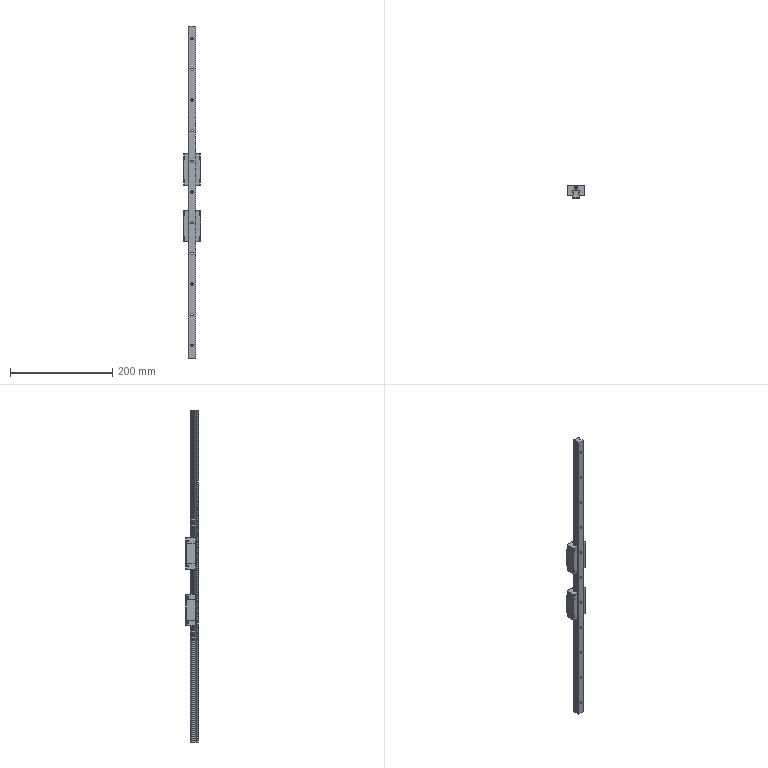Part | SolidWorks | 3 solids | 331 faces | box 34 x 24 x 650 mm | volume 182322 mm3 | plane 185 | cylinder 146 | commonest cylinder face diameters 0.8 x24 4 x24 4.5 x22 7.5 x22 3.3 x16 3.24 x12